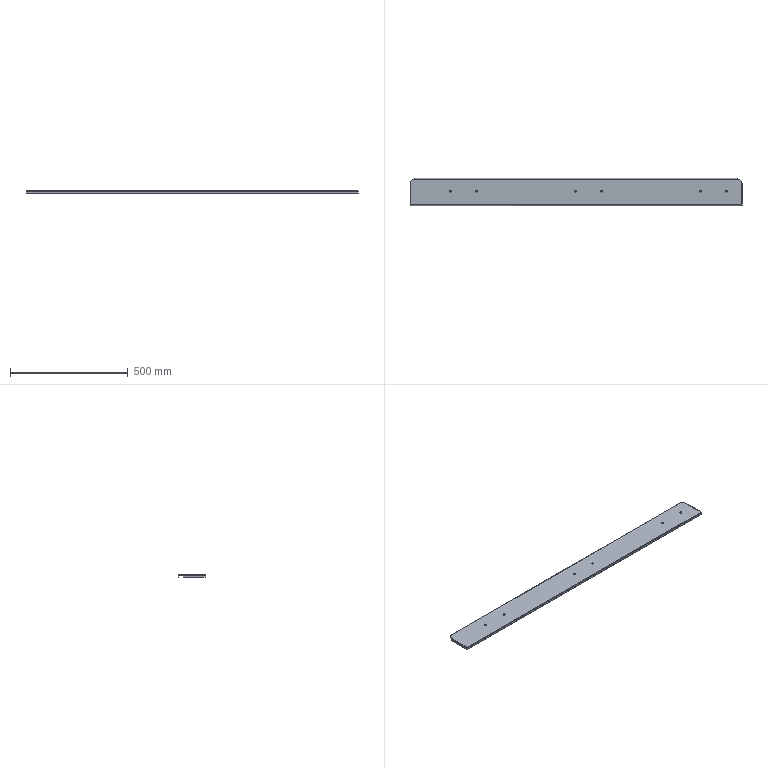Part | SolidWorks | features 3DProfileFeature 1, EdgeFlange 1, Fillet 1, FlatPattern 1, HoleWzd 1, LPattern 1, SMBaseFlange 1, SheetMetal 1 | 1 solid | 52 faces | box 1408 x 114.6 x 10 mm | volume 275844 mm3 | plane 26 | cone 12 | cylinder 10 | spline 4 | commonest cylinder face diameters 1.6 x4 4.6 x4 36 x2